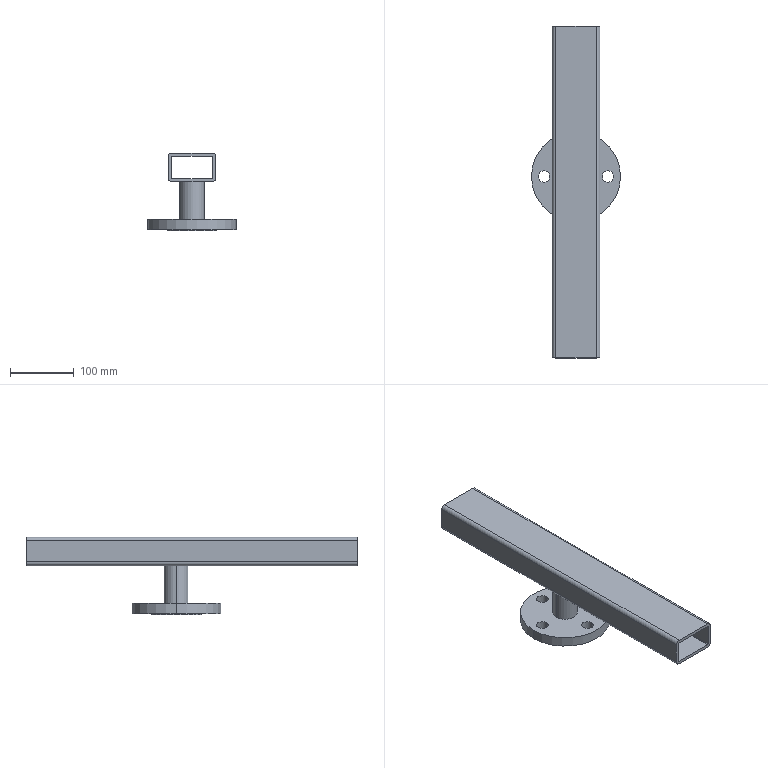Part | SolidWorks | features ICE 4, Extrusion 1 | 2 solids | 38 faces | box 140 x 521 x 122 mm | volume 862843 mm3 | cylinder 24 | plane 14 | commonest cylinder face diameters 18 x8 2 x4 12 x4 38 x2 39 x2 78 x2
STEP:
#1=CARTESIAN_POINT('',(-31.5,285.,-114.722));
#2=VERTEX_POINT('',#1);
#3=CARTESIAN_POINT('',(6.5,285.,-114.722));
#4=VERTEX_POINT('',#3);
#5=CARTESIAN_POINT('',(-12.5,285.,-114.722));
#6=DIRECTION('',(0.,0.,-1.));
#7=DIRECTION('',(-1.,0.,0.));
#8=AXIS2_PLACEMENT_3D('',#5,#6,#7);
#9=CIRCLE('',#8,19.);
#10=EDGE_CURVE('',#2,#4,#9,.T.);
#11=ORIENTED_EDGE('',*,*,#10,.F.);
#12=CARTESIAN_POINT('',(-31.5,285.,-37.722));
#13=VERTEX_POINT('',#12);
#14=CARTESIAN_POINT('',(-31.5,285.,-112.722));
#15=DIRECTION('',(0.,0.,1.));
#16=VECTOR('',#15,1000.);
#17=LINE('',#14,#16);
#18=EDGE_CURVE('',#2,#13,#17,.T.);
#19=ORIENTED_EDGE('',*,*,#18,.T.);
#20=CARTESIAN_POINT('',(6.5,285.,-37.722));
#21=VERTEX_POINT('',#20);
#22=CARTESIAN_POINT('',(-12.5,285.,-37.722));
#23=DIRECTION('',(0.,0.,-1.));
#24=DIRECTION('',(1.,0.,0.));
#25=AXIS2_PLACEMENT_3D('',#22,#23,#24);
#26=CIRCLE('',#25,19.);
#27=EDGE_CURVE('',#13,#21,#26,.T.);
#28=ORIENTED_EDGE('',*,*,#27,.T.);
#29=CARTESIAN_POINT('',(6.5,285.,-112.722));
#30=DIRECTION('',(0.,0.,1.));
#31=VECTOR('',#30,1000.);
#32=LINE('',#29,#31);
#33=EDGE_CURVE('',#4,#21,#32,.T.);
#34=ORIENTED_EDGE('',*,*,#33,.F.);
#35=EDGE_LOOP('',(#11,#19,#28,#34));
#36=FACE_OUTER_BOUND('',#35,.T.);
#37=CARTESIAN_POINT('',(-12.5,285.,-112.722));
#38=DIRECTION('',(0.,0.,1.));
#39=DIRECTION('',(1.,0.,0.));
#40=AXIS2_PLACEMENT_3D('',#37,#38,#39);
#41=CYLINDRICAL_SURFACE('',#40,19.);
#42=ADVANCED_FACE('',(#36),#41,.T.);
#43=CARTESIAN_POINT('',(-12.5,285.,-37.722));
#44=DIRECTION('',(0.,0.,-1.));
#45=DIRECTION('',(1.,0.,0.));
#46=AXIS2_PLACEMENT_3D('',#43,#44,#45);
#47=CIRCLE('',#46,19.);
#48=EDGE_CURVE('',#21,#13,#47,.T.);
#49=ORIENTED_EDGE('',*,*,#48,.F.);
#50=ORIENTED_EDGE('',*,*,#27,.F.);
#51=EDGE_LOOP('',(#49,#50));
#52=FACE_BOUND('',#51,.T.);
#53=CARTESIAN_POINT('',(19.,0.,-37.722));
#54=VERTEX_POINT('',#53);
#55=CARTESIAN_POINT('',(-44.,0.,-37.722));
#56=VERTEX_POINT('',#55);
#57=CARTESIAN_POINT('',(-44.,0.,-37.722));
#58=DIRECTION('',(-1.,0.,0.));
#59=VECTOR('',#58,1000.);
#60=LINE('',#57,#59);
#61=EDGE_CURVE('',#54,#56,#60,.T.);
#62=ORIENTED_EDGE('',*,*,#61,.T.);
#63=CARTESIAN_POINT('',(-44.,521.,-37.722));
#64=VERTEX_POINT('',#63);
#65=CARTESIAN_POINT('',(-44.,521.,-37.722));
#66=DIRECTION('',(0.,-1.,0.));
#67=VECTOR('',#66,1000.);
#68=LINE('',#65,#67);
#69=EDGE_CURVE('',#64,#56,#68,.T.);
#70=ORIENTED_EDGE('',*,*,#69,.F.);
#71=CARTESIAN_POINT('',(19.,521.,-37.722));
#72=VERTEX_POINT('',#71);
#73=CARTESIAN_POINT('',(-44.,521.,-37.722));
#74=DIRECTION('',(-1.,0.,0.));
#75=VECTOR('',#74,1000.);
#76=LINE('',#73,#75);
#77=EDGE_CURVE('',#72,#64,#76,.T.);
#78=ORIENTED_EDGE('',*,*,#77,.F.);
#79=CARTESIAN_POINT('',(19.,521.,-37.722));
#80=DIRECTION('',(0.,-1.,0.));
#81=VECTOR('',#80,1000.);
#82=LINE('',#79,#81);
#83=EDGE_CURVE('',#72,#54,#82,.T.);
#84=ORIENTED_EDGE('',*,*,#83,.T.);
#85=EDGE_LOOP('',(#62,#70,#78,#84));
#86=FACE_OUTER_BOUND('',#85,.T.);
#87=CARTESIAN_POINT('',(-44.,521.,-37.722));
#88=DIRECTION('',(0.,0.,1.));
#89=DIRECTION('',(1.,0.,0.));
#90=AXIS2_PLACEMENT_3D('',#87,#88,#89);
#91=PLANE('',#90);
#92=ADVANCED_FACE('',(#52,#86),#91,.F.);
#93=ORIENTED_EDGE('',*,*,#18,.F.);
#94=CARTESIAN_POINT('',(-12.5,285.,-114.722));
#95=DIRECTION('',(0.,0.,-1.));
#96=DIRECTION('',(-1.,0.,0.));
#97=AXIS2_PLACEMENT_3D('',#94,#95,#96);
#98=CIRCLE('',#97,19.);
#99=EDGE_CURVE('',#4,#2,#98,.T.);
#100=ORIENTED_EDGE('',*,*,#99,.F.);
#101=ORIENTED_EDGE('',*,*,#33,.T.);
#102=ORIENTED_EDGE('',*,*,#48,.T.);
#103=EDGE_LOOP('',(#93,#100,#101,#102));
#104=FACE_OUTER_BOUND('',#103,.T.);
#105=CARTESIAN_POINT('',(-12.5,285.,-112.722));
#106=DIRECTION('',(0.,0.,1.));
#107=DIRECTION('',(1.,0.,0.));
#108=AXIS2_PLACEMENT_3D('',#105,#106,#107);
#109=CYLINDRICAL_SURFACE('',#108,19.);
#110=ADVANCED_FACE('',(#104),#109,.T.);
#111=CARTESIAN_POINT('',(-50.,521.,1.278));
#112=VERTEX_POINT('',#111);
#113=CARTESIAN_POINT('',(-44.,521.,7.278));
#114=VERTEX_POINT('',#113);
#115=CARTESIAN_POINT('',(-44.,521.,1.278));
#116=DIRECTION('',(0.,1.,0.));
#117=DIRECTION('',(0.,0.,-1.));
#118=AXIS2_PLACEMENT_3D('',#115,#116,#117);
#119=CIRCLE('',#118,6.);
#120=EDGE_CURVE('',#112,#114,#119,.T.);
#121=ORIENTED_EDGE('',*,*,#120,.T.);
#122=CARTESIAN_POINT('',(19.,521.,7.278));
#123=VERTEX_POINT('',#122);
#124=CARTESIAN_POINT('',(-44.,521.,7.278));
#125=DIRECTION('',(1.,0.,0.));
#126=VECTOR('',#125,1000.);
#127=LINE('',#124,#126);
#128=EDGE_CURVE('',#114,#123,#127,.T.);
#129=ORIENTED_EDGE('',*,*,#128,.T.);
#130=CARTESIAN_POINT('',(25.,521.,1.278));
#131=VERTEX_POINT('',#130);
#132=CARTESIAN_POINT('',(19.,521.,1.278));
#133=DIRECTION('',(0.,1.,0.));
#134=DIRECTION('',(0.,0.,1.));
#135=AXIS2_PLACEMENT_3D('',#132,#133,#134);
#136=CIRCLE('',#135,6.);
#137=EDGE_CURVE('',#123,#131,#136,.T.);
#138=ORIENTED_EDGE('',*,*,#137,.T.);
#139=CARTESIAN_POINT('',(25.,521.,-31.722));
#140=VERTEX_POINT('',#139);
#141=CARTESIAN_POINT('',(25.,521.,1.278));
#142=DIRECTION('',(0.,0.,-1.));
#143=VECTOR('',#142,1000.);
#144=LINE('',#141,#143);
#145=EDGE_CURVE('',#131,#140,#144,.T.);
#146=ORIENTED_EDGE('',*,*,#145,.T.);
#147=CARTESIAN_POINT('',(19.,521.,-31.722));
#148=DIRECTION('',(0.,1.,0.));
#149=DIRECTION('',(0.,0.,-1.));
#150=AXIS2_PLACEMENT_3D('',#147,#148,#149);
#151=CIRCLE('',#150,6.);
#152=EDGE_CURVE('',#140,#72,#151,.T.);
#153=ORIENTED_EDGE('',*,*,#152,.T.);
#154=ORIENTED_EDGE('',*,*,#77,.T.);
#155=CARTESIAN_POINT('',(-50.,521.,-31.722));
#156=VERTEX_POINT('',#155);
#157=CARTESIAN_POINT('',(-44.,521.,-31.722));
#158=DIRECTION('',(0.,1.,0.));
#159=DIRECTION('',(0.,0.,-1.));
#160=AXIS2_PLACEMENT_3D('',#157,#158,#159);
#161=CIRCLE('',#160,6.);
#162=EDGE_CURVE('',#64,#156,#161,.T.);
#163=ORIENTED_EDGE('',*,*,#162,.T.);
#164=CARTESIAN_POINT('',(-50.,521.,1.278));
#165=DIRECTION('',(0.,0.,1.));
#166=VECTOR('',#165,1000.);
#167=LINE('',#164,#166);
#168=EDGE_CURVE('',#156,#112,#167,.T.);
#169=ORIENTED_EDGE('',*,*,#168,.T.);
#170=EDGE_LOOP('',(#121,#129,#138,#146,#153,#154,#163,#169));
#171=FACE_OUTER_BOUND('',#170,.T.);
#172=CARTESIAN_POINT('',(-45.,521.,1.278));
#173=VERTEX_POINT('',#172);
#174=CARTESIAN_POINT('',(-44.,521.,2.278));
#175=VERTEX_POINT('',#174);
#176=CARTESIAN_POINT('',(-44.,521.,1.278));
#177=DIRECTION('',(0.,1.,0.));
#178=DIRECTION('',(0.,0.,-1.));
#179=AXIS2_PLACEMENT_3D('',#176,#177,#178);
#180=CIRCLE('',#179,1.);
#181=EDGE_CURVE('',#173,#175,#180,.T.);
#182=ORIENTED_EDGE('',*,*,#181,.F.);
#183=CARTESIAN_POINT('',(-45.,521.,-31.722));
#184=VERTEX_POINT('',#183);
#185=CARTESIAN_POINT('',(-45.,521.,1.278));
#186=DIRECTION('',(0.,0.,1.));
#187=VECTOR('',#186,1000.);
#188=LINE('',#185,#187);
#189=EDGE_CURVE('',#184,#173,#188,.T.);
#190=ORIENTED_EDGE('',*,*,#189,.F.);
#191=CARTESIAN_POINT('',(-44.,521.,-32.722));
#192=VERTEX_POINT('',#191);
#193=CARTESIAN_POINT('',(-44.,521.,-31.722));
#194=DIRECTION('',(0.,1.,0.));
#195=DIRECTION('',(0.,0.,-1.));
#196=AXIS2_PLACEMENT_3D('',#193,#194,#195);
#197=CIRCLE('',#196,1.);
#198=EDGE_CURVE('',#192,#184,#197,.T.);
#199=ORIENTED_EDGE('',*,*,#198,.F.);
#200=CARTESIAN_POINT('',(19.,521.,-32.722));
#201=VERTEX_POINT('',#200);
#202=CARTESIAN_POINT('',(-44.,521.,-32.722));
#203=DIRECTION('',(-1.,0.,0.));
#204=VECTOR('',#203,1000.);
#205=LINE('',#202,#204);
#206=EDGE_CURVE('',#201,#192,#205,.T.);
#207=ORIENTED_EDGE('',*,*,#206,.F.);
#208=CARTESIAN_POINT('',(20.,521.,-31.722));
#209=VERTEX_POINT('',#208);
#210=CARTESIAN_POINT('',(19.,521.,-31.722));
#211=DIRECTION('',(0.,1.,0.));
#212=DIRECTION('',(0.,0.,-1.));
#213=AXIS2_PLACEMENT_3D('',#210,#211,#212);
#214=CIRCLE('',#213,1.);
#215=EDGE_CURVE('',#209,#201,#214,.T.);
#216=ORIENTED_EDGE('',*,*,#215,.F.);
#217=CARTESIAN_POINT('',(20.,521.,1.278));
#218=VERTEX_POINT('',#217);
#219=CARTESIAN_POINT('',(20.,521.,1.278));
#220=DIRECTION('',(0.,0.,-1.));
#221=VECTOR('',#220,1000.);
#222=LINE('',#219,#221);
#223=EDGE_CURVE('',#218,#209,#222,.T.);
#224=ORIENTED_EDGE('',*,*,#223,.F.);
#225=CARTESIAN_POINT('',(19.,521.,2.278));
#226=VERTEX_POINT('',#225);
#227=CARTESIAN_POINT('',(19.,521.,1.278));
#228=DIRECTION('',(0.,1.,0.));
#229=DIRECTION('',(0.,0.,1.));
#230=AXIS2_PLACEMENT_3D('',#227,#228,#229);
#231=CIRCLE('',#230,1.);
#232=EDGE_CURVE('',#226,#218,#231,.T.);
#233=ORIENTED_EDGE('',*,*,#232,.F.);
#234=CARTESIAN_POINT('',(-44.,521.,2.278));
#235=DIRECTION('',(1.,0.,0.));
#236=VECTOR('',#235,1000.);
#237=LINE('',#234,#236);
#238=EDGE_CURVE('',#175,#226,#237,.T.);
#239=ORIENTED_EDGE('',*,*,#238,.F.);
#240=EDGE_LOOP('',(#182,#190,#199,#207,#216,#224,#233,#239));
#241=FACE_BOUND('',#240,.T.);
#242=CARTESIAN_POINT('',(-44.,521.,1.278));
#243=DIRECTION('',(0.,-1.,0.));
#244=DIRECTION('',(0.,0.,-1.));
#245=AXIS2_PLACEMENT_3D('',#242,#243,#244);
#246=PLANE('',#245);
#247=ADVANCED_FACE('',(#171,#241),#246,.F.);
#248=CARTESIAN_POINT('',(-50.,0.,1.278));
#249=VERTEX_POINT('',#248);
#250=CARTESIAN_POINT('',(-44.,0.,7.278));
#251=VERTEX_POINT('',#250);
#252=CARTESIAN_POINT('',(-44.,0.,1.278));
#253=DIRECTION('',(0.,1.,0.));
#254=DIRECTION('',(0.,0.,-1.));
#255=AXIS2_PLACEMENT_3D('',#252,#253,#254);
#256=CIRCLE('',#255,6.);
#257=EDGE_CURVE('',#249,#251,#256,.T.);
#258=ORIENTED_EDGE('',*,*,#257,.F.);
#259=CARTESIAN_POINT('',(-50.,0.,-31.722));
#260=VERTEX_POINT('',#259);
#261=CARTESIAN_POINT('',(-50.,0.,1.278));
#262=DIRECTION('',(0.,0.,1.));
#263=VECTOR('',#262,1000.);
#264=LINE('',#261,#263);
#265=EDGE_CURVE('',#260,#249,#264,.T.);
#266=ORIENTED_EDGE('',*,*,#265,.F.);
#267=CARTESIAN_POINT('',(-44.,0.,-31.722));
#268=DIRECTION('',(0.,1.,0.));
#269=DIRECTION('',(0.,0.,-1.));
#270=AXIS2_PLACEMENT_3D('',#267,#268,#269);
#271=CIRCLE('',#270,6.);
#272=EDGE_CURVE('',#56,#260,#271,.T.);
#273=ORIENTED_EDGE('',*,*,#272,.F.);
#274=ORIENTED_EDGE('',*,*,#61,.F.);
#275=CARTESIAN_POINT('',(25.,0.,-31.722));
#276=VERTEX_POINT('',#275);
#277=CARTESIAN_POINT('',(19.,0.,-31.722));
#278=DIRECTION('',(0.,1.,0.));
#279=DIRECTION('',(0.,0.,-1.));
#280=AXIS2_PLACEMENT_3D('',#277,#278,#279);
#281=CIRCLE('',#280,6.);
#282=EDGE_CURVE('',#276,#54,#281,.T.);
#283=ORIENTED_EDGE('',*,*,#282,.F.);
#284=CARTESIAN_POINT('',(25.,0.,1.278));
#285=VERTEX_POINT('',#284);
#286=CARTESIAN_POINT('',(25.,0.,1.278));
#287=DIRECTION('',(0.,0.,-1.));
#288=VECTOR('',#287,1000.);
#289=LINE('',#286,#288);
#290=EDGE_CURVE('',#285,#276,#289,.T.);
#291=ORIENTED_EDGE('',*,*,#290,.F.);
#292=CARTESIAN_POINT('',(19.,0.,7.278));
#293=VERTEX_POINT('',#292);
#294=CARTESIAN_POINT('',(19.,0.,1.278));
#295=DIRECTION('',(0.,1.,0.));
#296=DIRECTION('',(0.,0.,1.));
#297=AXIS2_PLACEMENT_3D('',#294,#295,#296);
#298=CIRCLE('',#297,6.);
#299=EDGE_CURVE('',#293,#285,#298,.T.);
#300=ORIENTED_EDGE('',*,*,#299,.F.);
#301=CARTESIAN_POINT('',(-44.,0.,7.278));
#302=DIRECTION('',(1.,0.,0.));
#303=VECTOR('',#302,1000.);
#304=LINE('',#301,#303);
#305=EDGE_CURVE('',#251,#293,#304,.T.);
#306=ORIENTED_EDGE('',*,*,#305,.F.);
#307=EDGE_LOOP('',(#258,#266,#273,#274,#283,#291,#300,#306));
#308=FACE_OUTER_BOUND('',#307,.T.);
#309=CARTESIAN_POINT('',(-45.,0.,-31.722));
#310=VERTEX_POINT('',#309);
#311=CARTESIAN_POINT('',(-45.,0.,1.278));
#312=VERTEX_POINT('',#311);
#313=CARTESIAN_POINT('',(-45.,0.,1.278));
#314=DIRECTION('',(0.,0.,1.));
#315=VECTOR('',#314,1000.);
#316=LINE('',#313,#315);
#317=EDGE_CURVE('',#310,#312,#316,.T.);
#318=ORIENTED_EDGE('',*,*,#317,.T.);
#319=CARTESIAN_POINT('',(-44.,0.,2.278));
#320=VERTEX_POINT('',#319);
#321=CARTESIAN_POINT('',(-44.,0.,1.278));
#322=DIRECTION('',(0.,1.,0.));
#323=DIRECTION('',(0.,0.,-1.));
#324=AXIS2_PLACEMENT_3D('',#321,#322,#323);
#325=CIRCLE('',#324,1.);
#326=EDGE_CURVE('',#312,#320,#325,.T.);
#327=ORIENTED_EDGE('',*,*,#326,.T.);
#328=CARTESIAN_POINT('',(19.,0.,2.278));
#329=VERTEX_POINT('',#328);
#330=CARTESIAN_POINT('',(-44.,0.,2.278));
#331=DIRECTION('',(1.,0.,0.));
#332=VECTOR('',#331,1000.);
#333=LINE('',#330,#332);
#334=EDGE_CURVE('',#320,#329,#333,.T.);
#335=ORIENTED_EDGE('',*,*,#334,.T.);
#336=CARTESIAN_POINT('',(20.,0.,1.278));
#337=VERTEX_POINT('',#336);
#338=CARTESIAN_POINT('',(19.,0.,1.278));
#339=DIRECTION('',(0.,1.,0.));
#340=DIRECTION('',(0.,0.,1.));
#341=AXIS2_PLACEMENT_3D('',#338,#339,#340);
#342=CIRCLE('',#341,1.);
#343=EDGE_CURVE('',#329,#337,#342,.T.);
#344=ORIENTED_EDGE('',*,*,#343,.T.);
#345=CARTESIAN_POINT('',(20.,0.,-31.722));
#346=VERTEX_POINT('',#345);
#347=CARTESIAN_POINT('',(20.,0.,1.278));
#348=DIRECTION('',(0.,0.,-1.));
#349=VECTOR('',#348,1000.);
#350=LINE('',#347,#349);
#351=EDGE_CURVE('',#337,#346,#350,.T.);
#352=ORIENTED_EDGE('',*,*,#351,.T.);
#353=CARTESIAN_POINT('',(19.,0.,-32.722));
#354=VERTEX_POINT('',#353);
#355=CARTESIAN_POINT('',(19.,0.,-31.722));
#356=DIRECTION('',(0.,1.,0.));
#357=DIRECTION('',(0.,0.,-1.));
#358=AXIS2_PLACEMENT_3D('',#355,#356,#357);
#359=CIRCLE('',#358,1.);
#360=EDGE_CURVE('',#346,#354,#359,.T.);
#361=ORIENTED_EDGE('',*,*,#360,.T.);
#362=CARTESIAN_POINT('',(-44.,0.,-32.722));
#363=VERTEX_POINT('',#362);
#364=CARTESIAN_POINT('',(-44.,0.,-32.722));
#365=DIRECTION('',(-1.,0.,0.));
#366=VECTOR('',#365,1000.);
#367=LINE('',#364,#366);
#368=EDGE_CURVE('',#354,#363,#367,.T.);
#369=ORIENTED_EDGE('',*,*,#368,.T.);
#370=CARTESIAN_POINT('',(-44.,0.,-31.722));
#371=DIRECTION('',(0.,1.,0.));
#372=DIRECTION('',(0.,0.,-1.));
#373=AXIS2_PLACEMENT_3D('',#370,#371,#372);
#374=CIRCLE('',#373,1.);
#375=EDGE_CURVE('',#363,#310,#374,.T.);
#376=ORIENTED_EDGE('',*,*,#375,.T.);
#377=EDGE_LOOP('',(#318,#327,#335,#344,#352,#361,#369,#376));
#378=FACE_BOUND('',#377,.T.);
#379=CARTESIAN_POINT('',(-44.,0.,1.278));
#380=DIRECTION('',(0.,-1.,0.));
#381=DIRECTION('',(0.,0.,-1.));
#382=AXIS2_PLACEMENT_3D('',#379,#380,#381);
#383=PLANE('',#382);
#384=ADVANCED_FACE('',(#308,#378),#383,.T.);
#385=ORIENTED_EDGE('',*,*,#257,.T.);
#386=CARTESIAN_POINT('',(-44.,521.,7.278));
#387=DIRECTION('',(0.,-1.,0.));
#388=VECTOR('',#387,1000.);
#389=LINE('',#386,#388);
#390=EDGE_CURVE('',#114,#251,#389,.T.);
#391=ORIENTED_EDGE('',*,*,#390,.F.);
#392=ORIENTED_EDGE('',*,*,#120,.F.);
#393=CARTESIAN_POINT('',(-50.,521.,1.278));
#394=DIRECTION('',(0.,-1.,0.));
#395=VECTOR('',#394,1000.);
#396=LINE('',#393,#395);
#397=EDGE_CURVE('',#112,#249,#396,.T.);
#398=ORIENTED_EDGE('',*,*,#397,.T.);
#399=EDGE_LOOP('',(#385,#391,#392,#398));
#400=FACE_OUTER_BOUND('',#399,.T.);
#401=CARTESIAN_POINT('',(-44.,521.,1.278));
#402=DIRECTION('',(0.,-1.,0.));
#403=DIRECTION('',(0.,0.,-1.));
#404=AXIS2_PLACEMENT_3D('',#401,#402,#403);
#405=CYLINDRICAL_SURFACE('',#404,6.);
#406=ADVANCED_FACE('',(#400),#405,.T.);
#407=ORIENTED_EDGE('',*,*,#305,.T.);
#408=CARTESIAN_POINT('',(19.,521.,7.278));
#409=DIRECTION('',(0.,-1.,0.));
#410=VECTOR('',#409,1000.);
#411=LINE('',#408,#410);
#412=EDGE_CURVE('',#123,#293,#411,.T.);
#413=ORIENTED_EDGE('',*,*,#412,.F.);
#414=ORIENTED_EDGE('',*,*,#128,.F.);
#415=ORIENTED_EDGE('',*,*,#390,.T.);
#416=EDGE_LOOP('',(#407,#413,#414,#415));
#417=FACE_OUTER_BOUND('',#416,.T.);
#418=CARTESIAN_POINT('',(-44.,521.,7.278));
#419=DIRECTION('',(0.,0.,-1.));
#420=DIRECTION('',(-1.,0.,0.));
#421=AXIS2_PLACEMENT_3D('',#418,#419,#420);
#422=PLANE('',#421);
#423=ADVANCED_FACE('',(#417),#422,.F.);
#424=ORIENTED_EDGE('',*,*,#299,.T.);
#425=CARTESIAN_POINT('',(25.,521.,1.278));
#426=DIRECTION('',(0.,-1.,0.));
#427=VECTOR('',#426,1000.);
#428=LINE('',#425,#427);
#429=EDGE_CURVE('',#131,#285,#428,.T.);
#430=ORIENTED_EDGE('',*,*,#429,.F.);
#431=ORIENTED_EDGE('',*,*,#137,.F.);
#432=ORIENTED_EDGE('',*,*,#412,.T.);
#433=EDGE_LOOP('',(#424,#430,#431,#432));
#434=FACE_OUTER_BOUND('',#433,.T.);
#435=CARTESIAN_POINT('',(19.,521.,1.278));
#436=DIRECTION('',(0.,-1.,0.));
#437=DIRECTION('',(0.,0.,-1.));
#438=AXIS2_PLACEMENT_3D('',#435,#436,#437);
#439=CYLINDRICAL_SURFACE('',#438,6.);
#440=ADVANCED_FACE('',(#434),#439,.T.);
#441=ORIENTED_EDGE('',*,*,#290,.T.);
#442=CARTESIAN_POINT('',(25.,521.,-31.722));
#443=DIRECTION('',(0.,-1.,0.));
#444=VECTOR('',#443,1000.);
#445=LINE('',#442,#444);
#446=EDGE_CURVE('',#140,#276,#445,.T.);
#447=ORIENTED_EDGE('',*,*,#446,.F.);
#448=ORIENTED_EDGE('',*,*,#145,.F.);
#449=ORIENTED_EDGE('',*,*,#429,.T.);
#450=EDGE_LOOP('',(#441,#447,#448,#449));
#451=FACE_OUTER_BOUND('',#450,.T.);
#452=CARTESIAN_POINT('',(25.,521.,1.278));
#453=DIRECTION('',(-1.,0.,0.));
#454=DIRECTION('',(0.,0.,1.));
#455=AXIS2_PLACEMENT_3D('',#452,#453,#454);
#456=PLANE('',#455);
#457=ADVANCED_FACE('',(#451),#456,.F.);
#458=ORIENTED_EDGE('',*,*,#282,.T.);
#459=ORIENTED_EDGE('',*,*,#83,.F.);
#460=ORIENTED_EDGE('',*,*,#152,.F.);
#461=ORIENTED_EDGE('',*,*,#446,.T.);
#462=EDGE_LOOP('',(#458,#459,#460,#461));
#463=FACE_OUTER_BOUND('',#462,.T.);
#464=CARTESIAN_POINT('',(19.,521.,-31.722));
#465=DIRECTION('',(0.,-1.,0.));
#466=DIRECTION('',(0.,0.,-1.));
#467=AXIS2_PLACEMENT_3D('',#464,#465,#466);
#468=CYLINDRICAL_SURFACE('',#467,6.);
#469=ADVANCED_FACE('',(#463),#468,.T.);
#470=ORIENTED_EDGE('',*,*,#272,.T.);
#471=CARTESIAN_POINT('',(-50.,521.,-31.722));
#472=DIRECTION('',(0.,-1.,0.));
#473=VECTOR('',#472,1000.);
#474=LINE('',#471,#473);
#475=EDGE_CURVE('',#156,#260,#474,.T.);
#476=ORIENTED_EDGE('',*,*,#475,.F.);
#477=ORIENTED_EDGE('',*,*,#162,.F.);
#478=ORIENTED_EDGE('',*,*,#69,.T.);
#479=EDGE_LOOP('',(#470,#476,#477,#478));
#480=FACE_OUTER_BOUND('',#479,.T.);
#481=CARTESIAN_POINT('',(-44.,521.,-31.722));
#482=DIRECTION('',(0.,-1.,0.));
#483=DIRECTION('',(0.,0.,-1.));
#484=AXIS2_PLACEMENT_3D('',#481,#482,#483);
#485=CYLINDRICAL_SURFACE('',#484,6.);
#486=ADVANCED_FACE('',(#480),#485,.T.);
#487=ORIENTED_EDGE('',*,*,#265,.T.);
#488=ORIENTED_EDGE('',*,*,#397,.F.);
#489=ORIENTED_EDGE('',*,*,#168,.F.);
#490=ORIENTED_EDGE('',*,*,#475,.T.);
#491=EDGE_LOOP('',(#487,#488,#489,#490));
#492=FACE_OUTER_BOUND('',#491,.T.);
#493=CARTESIAN_POINT('',(-50.,521.,1.278));
#494=DIRECTION('',(1.,0.,0.));
#495=DIRECTION('',(0.,0.,-1.));
#496=AXIS2_PLACEMENT_3D('',#493,#494,#495);
#497=PLANE('',#496);
#498=ADVANCED_FACE('',(#492),#497,.F.);
#499=ORIENTED_EDGE('',*,*,#326,.F.);
#500=CARTESIAN_POINT('',(-45.,521.,1.278));
#501=DIRECTION('',(0.,-1.,0.));
#502=VECTOR('',#501,1000.);
#503=LINE('',#500,#502);
#504=EDGE_CURVE('',#173,#312,#503,.T.);
#505=ORIENTED_EDGE('',*,*,#504,.F.);
#506=ORIENTED_EDGE('',*,*,#181,.T.);
#507=CARTESIAN_POINT('',(-44.,521.,2.278));
#508=DIRECTION('',(0.,-1.,0.));
#509=VECTOR('',#508,1000.);
#510=LINE('',#507,#509);
#511=EDGE_CURVE('',#175,#320,#510,.T.);
#512=ORIENTED_EDGE('',*,*,#511,.T.);
#513=EDGE_LOOP('',(#499,#505,#506,#512));
#514=FACE_OUTER_BOUND('',#513,.T.);
#515=CARTESIAN_POINT('',(-44.,521.,1.278));
#516=DIRECTION('',(0.,-1.,0.));
#517=DIRECTION('',(0.,0.,-1.));
#518=AXIS2_PLACEMENT_3D('',#515,#516,#517);
#519=CYLINDRICAL_SURFACE('',#518,1.);
#520=ADVANCED_FACE('',(#514),#519,.F.);
#521=ORIENTED_EDGE('',*,*,#334,.F.);
#522=ORIENTED_EDGE('',*,*,#511,.F.);
#523=ORIENTED_EDGE('',*,*,#238,.T.);
#524=CARTESIAN_POINT('',(19.,521.,2.278));
#525=DIRECTION('',(0.,-1.,0.));
#526=VECTOR('',#525,1000.);
#527=LINE('',#524,#526);
#528=EDGE_CURVE('',#226,#329,#527,.T.);
#529=ORIENTED_EDGE('',*,*,#528,.T.);
#530=EDGE_LOOP('',(#521,#522,#523,#529));
#531=FACE_OUTER_BOUND('',#530,.T.);
#532=CARTESIAN_POINT('',(-44.,521.,2.278));
#533=DIRECTION('',(0.,0.,-1.));
#534=DIRECTION('',(-1.,0.,0.));
#535=AXIS2_PLACEMENT_3D('',#532,#533,#534);
#536=PLANE('',#535);
#537=ADVANCED_FACE('',(#531),#536,.T.);
#538=ORIENTED_EDGE('',*,*,#343,.F.);
#539=ORIENTED_EDGE('',*,*,#528,.F.);
#540=ORIENTED_EDGE('',*,*,#232,.T.);
#541=CARTESIAN_POINT('',(20.,521.,1.278));
#542=DIRECTION('',(0.,-1.,0.));
#543=VECTOR('',#542,1000.);
#544=LINE('',#541,#543);
#545=EDGE_CURVE('',#218,#337,#544,.T.);
#546=ORIENTED_EDGE('',*,*,#545,.T.);
#547=EDGE_LOOP('',(#538,#539,#540,#546));
#548=FACE_OUTER_BOUND('',#547,.T.);
#549=CARTESIAN_POINT('',(19.,521.,1.278));
#550=DIRECTION('',(0.,-1.,0.));
#551=DIRECTION('',(0.,0.,-1.));
#552=AXIS2_PLACEMENT_3D('',#549,#550,#551);
#553=CYLINDRICAL_SURFACE('',#552,1.);
#554=ADVANCED_FACE('',(#548),#553,.F.);
#555=ORIENTED_EDGE('',*,*,#351,.F.);
#556=ORIENTED_EDGE('',*,*,#545,.F.);
#557=ORIENTED_EDGE('',*,*,#223,.T.);
#558=CARTESIAN_POINT('',(20.,521.,-31.722));
#559=DIRECTION('',(0.,-1.,0.));
#560=VECTOR('',#559,1000.);
#561=LINE('',#558,#560);
#562=EDGE_CURVE('',#209,#346,#561,.T.);
#563=ORIENTED_EDGE('',*,*,#562,.T.);
#564=EDGE_LOOP('',(#555,#556,#557,#563));
#565=FACE_OUTER_BOUND('',#564,.T.);
#566=CARTESIAN_POINT('',(20.,521.,1.278));
#567=DIRECTION('',(-1.,0.,0.));
#568=DIRECTION('',(0.,0.,1.));
#569=AXIS2_PLACEMENT_3D('',#566,#567,#568);
#570=PLANE('',#569);
#571=ADVANCED_FACE('',(#565),#570,.T.);
#572=ORIENTED_EDGE('',*,*,#360,.F.);
#573=ORIENTED_EDGE('',*,*,#562,.F.);
#574=ORIENTED_EDGE('',*,*,#215,.T.);
#575=CARTESIAN_POINT('',(19.,521.,-32.722));
#576=DIRECTION('',(0.,-1.,0.));
#577=VECTOR('',#576,1000.);
#578=LINE('',#575,#577);
#579=EDGE_CURVE('',#201,#354,#578,.T.);
#580=ORIENTED_EDGE('',*,*,#579,.T.);
#581=EDGE_LOOP('',(#572,#573,#574,#580));
#582=FACE_OUTER_BOUND('',#581,.T.);
#583=CARTESIAN_POINT('',(19.,521.,-31.722));
#584=DIRECTION('',(0.,-1.,0.));
#585=DIRECTION('',(0.,0.,-1.));
#586=AXIS2_PLACEMENT_3D('',#583,#584,#585);
#587=CYLINDRICAL_SURFACE('',#586,1.);
#588=ADVANCED_FACE('',(#582),#587,.F.);
#589=ORIENTED_EDGE('',*,*,#368,.F.);
#590=ORIENTED_EDGE('',*,*,#579,.F.);
#591=ORIENTED_EDGE('',*,*,#206,.T.);
#592=CARTESIAN_POINT('',(-44.,521.,-32.722));
#593=DIRECTION('',(0.,-1.,0.));
#594=VECTOR('',#593,1000.);
#595=LINE('',#592,#594);
#596=EDGE_CURVE('',#192,#363,#595,.T.);
#597=ORIENTED_EDGE('',*,*,#596,.T.);
#598=EDGE_LOOP('',(#589,#590,#591,#597));
#599=FACE_OUTER_BOUND('',#598,.T.);
#600=CARTESIAN_POINT('',(-44.,521.,-32.722));
#601=DIRECTION('',(0.,0.,1.));
#602=DIRECTION('',(1.,0.,0.));
#603=AXIS2_PLACEMENT_3D('',#600,#601,#602);
#604=PLANE('',#603);
#605=ADVANCED_FACE('',(#599),#604,.T.);
#606=ORIENTED_EDGE('',*,*,#375,.F.);
#607=ORIENTED_EDGE('',*,*,#596,.F.);
#608=ORIENTED_EDGE('',*,*,#198,.T.);
#609=CARTESIAN_POINT('',(-45.,521.,-31.722));
#610=DIRECTION('',(0.,-1.,0.));
#611=VECTOR('',#610,1000.);
#612=LINE('',#609,#611);
#613=EDGE_CURVE('',#184,#310,#612,.T.);
#614=ORIENTED_EDGE('',*,*,#613,.T.);
#615=EDGE_LOOP('',(#606,#607,#608,#614));
#616=FACE_OUTER_BOUND('',#615,.T.);
#617=CARTESIAN_POINT('',(-44.,521.,-31.722));
#618=DIRECTION('',(0.,-1.,0.));
#619=DIRECTION('',(0.,0.,-1.));
#620=AXIS2_PLACEMENT_3D('',#617,#618,#619);
#621=CYLINDRICAL_SURFACE('',#620,1.);
#622=ADVANCED_FACE('',(#616),#621,.F.);
#623=ORIENTED_EDGE('',*,*,#317,.F.);
#624=ORIENTED_EDGE('',*,*,#613,.F.);
#625=ORIENTED_EDGE('',*,*,#189,.T.);
#626=ORIENTED_EDGE('',*,*,#504,.T.);
#627=EDGE_LOOP('',(#623,#624,#625,#626));
#628=FACE_OUTER_BOUND('',#627,.T.);
#629=CARTESIAN_POINT('',(-45.,521.,1.278));
#630=DIRECTION('',(1.,0.,0.));
#631=DIRECTION('',(0.,0.,-1.));
#632=AXIS2_PLACEMENT_3D('',#629,#630,#631);
#633=PLANE('',#632);
#634=ADVANCED_FACE('',(#628),#633,.T.);
#635=ORIENTED_EDGE('',*,*,#99,.T.);
#636=ORIENTED_EDGE('',*,*,#10,.T.);
#637=EDGE_LOOP('',(#635,#636));
#638=FACE_OUTER_BOUND('',#637,.T.);
#639=CARTESIAN_POINT('',(-12.5,285.,-114.722));
#640=DIRECTION('',(0.,0.,-1.));
#641=DIRECTION('',(-1.,0.,0.));
#642=AXIS2_PLACEMENT_3D('',#639,#640,#641);
#643=PLANE('',#642);
#644=ADVANCED_FACE('',(#638),#643,.T.);
#645=CLOSED_SHELL('',(#42,#92,#110,#247,#384,#406,#423,#440,#457,#469,#486,#498,#520,#537,#554,#571,#588,#605,#622,#634,#644));
#646=MANIFOLD_SOLID_BREP('',#645);
#647=CARTESIAN_POINT('',(7.,285.,-96.722));
#648=VERTEX_POINT('',#647);
#649=CARTESIAN_POINT('',(-32.,285.,-96.722));
#650=VERTEX_POINT('',#649);
#651=CARTESIAN_POINT('',(-12.5,285.,-96.722));
#652=DIRECTION('',(0.,0.,-1.));
#653=DIRECTION('',(-1.,0.,0.));
#654=AXIS2_PLACEMENT_3D('',#651,#652,#653);
#655=CIRCLE('',#654,19.5);
#656=EDGE_CURVE('',#648,#650,#655,.T.);
#657=ORIENTED_EDGE('',*,*,#656,.F.);
#658=CARTESIAN_POINT('',(7.,285.,-114.722));
#659=VERTEX_POINT('',#658);
#660=CARTESIAN_POINT('',(7.,285.,17.432));
#661=DIRECTION('',(0.,0.,-1.));
#662=VECTOR('',#661,1000.);
#663=LINE('',#660,#662);
#664=EDGE_CURVE('',#648,#659,#663,.T.);
#665=ORIENTED_EDGE('',*,*,#664,.T.);
#666=CARTESIAN_POINT('',(-32.,285.,-114.722));
#667=VERTEX_POINT('',#666);
#668=CARTESIAN_POINT('',(-12.5,285.,-114.722));
#669=DIRECTION('',(0.,0.,-1.));
#670=DIRECTION('',(-1.,0.,0.));
#671=AXIS2_PLACEMENT_3D('',#668,#669,#670);
#672=CIRCLE('',#671,19.5);
#673=EDGE_CURVE('',#659,#667,#672,.T.);
#674=ORIENTED_EDGE('',*,*,#673,.T.);
#675=CARTESIAN_POINT('',(-32.,285.,17.432));
#676=DIRECTION('',(0.,0.,-1.));
#677=VECTOR('',#676,1000.);
#678=LINE('',#675,#677);
#679=EDGE_CURVE('',#650,#667,#678,.T.);
#680=ORIENTED_EDGE('',*,*,#679,.F.);
#681=EDGE_LOOP('',(#657,#665,#674,#680));
#682=FACE_OUTER_BOUND('',#681,.T.);
#683=CARTESIAN_POINT('',(-12.5,285.,17.432));
#684=DIRECTION('',(0.,0.,-1.));
#685=DIRECTION('',(-1.,0.,0.));
#686=AXIS2_PLACEMENT_3D('',#683,#684,#685);
#687=CYLINDRICAL_SURFACE('',#686,19.5);
#688=ADVANCED_FACE('',(#682),#687,.F.);
#689=CARTESIAN_POINT('',(-51.5,285.,-114.722));
#690=VERTEX_POINT('',#689);
#691=CARTESIAN_POINT('',(26.5,285.,-114.722));
#692=VERTEX_POINT('',#691);
#693=CARTESIAN_POINT('',(-12.5,285.,-114.722));
#694=DIRECTION('',(0.,0.,-1.));
#695=DIRECTION('',(-1.,0.,0.));
#696=AXIS2_PLACEMENT_3D('',#693,#694,#695);
#697=CIRCLE('',#696,39.);
#698=EDGE_CURVE('',#690,#692,#697,.T.);
#699=ORIENTED_EDGE('',*,*,#698,.F.);
#700=CARTESIAN_POINT('',(-51.5,285.,-112.722));
#701=VERTEX_POINT('',#700);
#702=CARTESIAN_POINT('',(-51.5,285.,-114.722));
#703=DIRECTION('',(0.,0.,1.));
#704=VECTOR('',#703,1000.);
#705=LINE('',#702,#704);
#706=EDGE_CURVE('',#690,#701,#705,.T.);
#707=ORIENTED_EDGE('',*,*,#706,.T.);
#708=CARTESIAN_POINT('',(26.5,285.,-112.722));
#709=VERTEX_POINT('',#708);
#710=CARTESIAN_POINT('',(-12.5,285.,-112.722));
#711=DIRECTION('',(0.,0.,-1.));
#712=DIRECTION('',(-1.,0.,0.));
#713=AXIS2_PLACEMENT_3D('',#710,#711,#712);
#714=CIRCLE('',#713,39.);
#715=EDGE_CURVE('',#701,#709,#714,.T.);
#716=ORIENTED_EDGE('',*,*,#715,.T.);
#717=CARTESIAN_POINT('',(26.5,285.,-114.722));
#718=DIRECTION('',(0.,0.,1.));
#719=VECTOR('',#718,1000.);
#720=LINE('',#717,#719);
#721=EDGE_CURVE('',#692,#709,#720,.T.);
#722=ORIENTED_EDGE('',*,*,#721,.F.);
#723=EDGE_LOOP('',(#699,#707,#716,#722));
#724=FACE_OUTER_BOUND('',#723,.T.);
#725=CARTESIAN_POINT('',(-12.5,285.,-114.722));
#726=DIRECTION('',(0.,0.,1.));
#727=DIRECTION('',(1.,0.,0.));
#728=AXIS2_PLACEMENT_3D('',#725,#726,#727);
#729=CYLINDRICAL_SURFACE('',#728,39.);
#730=ADVANCED_FACE('',(#724),#729,.T.);
#731=CARTESIAN_POINT('',(46.5,285.,-96.722));
#732=VERTEX_POINT('',#731);
#733=CARTESIAN_POINT('',(28.5,285.,-96.722));
#734=VERTEX_POINT('',#733);
#735=CARTESIAN_POINT('',(37.5,285.,-96.722));
#736=DIRECTION('',(0.,0.,-1.));
#737=DIRECTION('',(-1.,0.,0.));
#738=AXIS2_PLACEMENT_3D('',#735,#736,#737);
#739=CIRCLE('',#738,9.);
#740=EDGE_CURVE('',#732,#734,#739,.T.);
#741=ORIENTED_EDGE('',*,*,#740,.F.);
#742=CARTESIAN_POINT('',(46.5,285.,-112.722));
#743=VERTEX_POINT('',#742);
#744=CARTESIAN_POINT('',(46.5,285.,-96.722));
#745=DIRECTION('',(0.,0.,-1.));
#746=VECTOR('',#745,1000.);
#747=LINE('',#744,#746);
#748=EDGE_CURVE('',#732,#743,#747,.T.);
#749=ORIENTED_EDGE('',*,*,#748,.T.);
#750=CARTESIAN_POINT('',(28.5,285.,-112.722));
#751=VERTEX_POINT('',#750);
#752=CARTESIAN_POINT('',(37.5,285.,-112.722));
#753=DIRECTION('',(0.,0.,-1.));
#754=DIRECTION('',(-1.,0.,0.));
#755=AXIS2_PLACEMENT_3D('',#752,#753,#754);
#756=CIRCLE('',#755,9.);
#757=EDGE_CURVE('',#743,#751,#756,.T.);
#758=ORIENTED_EDGE('',*,*,#757,.T.);
#759=CARTESIAN_POINT('',(28.5,285.,-96.722));
#760=DIRECTION('',(0.,0.,-1.));
#761=VECTOR('',#760,1000.);
#762=LINE('',#759,#761);
#763=EDGE_CURVE('',#734,#751,#762,.T.);
#764=ORIENTED_EDGE('',*,*,#763,.F.);
#765=EDGE_LOOP('',(#741,#749,#758,#764));
#766=FACE_OUTER_BOUND('',#765,.T.);
#767=CARTESIAN_POINT('',(37.5,285.,-96.722));
#768=DIRECTION('',(0.,0.,-1.));
#769=DIRECTION('',(-1.,0.,0.));
#770=AXIS2_PLACEMENT_3D('',#767,#768,#769);
#771=CYLINDRICAL_SURFACE('',#770,9.);
#772=ADVANCED_FACE('',(#766),#771,.F.);
#773=CARTESIAN_POINT('',(-3.5,235.,-96.722));
#774=VERTEX_POINT('',#773);
#775=CARTESIAN_POINT('',(-21.5,235.,-96.722));
#776=VERTEX_POINT('',#775);
#777=CARTESIAN_POINT('',(-12.5,235.,-96.722));
#778=DIRECTION('',(0.,0.,-1.));
#779=DIRECTION('',(-1.,0.,0.));
#780=AXIS2_PLACEMENT_3D('',#777,#778,#779);
#781=CIRCLE('',#780,9.);
#782=EDGE_CURVE('',#774,#776,#781,.T.);
#783=ORIENTED_EDGE('',*,*,#782,.F.);
#784=CARTESIAN_POINT('',(-3.5,235.,-112.722));
#785=VERTEX_POINT('',#784);
#786=CARTESIAN_POINT('',(-3.5,235.,-96.722));
#787=DIRECTION('',(0.,0.,-1.));
#788=VECTOR('',#787,1000.);
#789=LINE('',#786,#788);
#790=EDGE_CURVE('',#774,#785,#789,.T.);
#791=ORIENTED_EDGE('',*,*,#790,.T.);
#792=CARTESIAN_POINT('',(-21.5,235.,-112.722));
#793=VERTEX_POINT('',#792);
#794=CARTESIAN_POINT('',(-12.5,235.,-112.722));
#795=DIRECTION('',(0.,0.,-1.));
#796=DIRECTION('',(-1.,0.,0.));
#797=AXIS2_PLACEMENT_3D('',#794,#795,#796);
#798=CIRCLE('',#797,9.);
#799=EDGE_CURVE('',#785,#793,#798,.T.);
#800=ORIENTED_EDGE('',*,*,#799,.T.);
#801=CARTESIAN_POINT('',(-21.5,235.,-96.722));
#802=DIRECTION('',(0.,0.,-1.));
#803=VECTOR('',#802,1000.);
#804=LINE('',#801,#803);
#805=EDGE_CURVE('',#776,#793,#804,.T.);
#806=ORIENTED_EDGE('',*,*,#805,.F.);
#807=EDGE_LOOP('',(#783,#791,#800,#806));
#808=FACE_OUTER_BOUND('',#807,.T.);
#809=CARTESIAN_POINT('',(-12.5,235.,-96.722));
#810=DIRECTION('',(0.,0.,-1.));
#811=DIRECTION('',(-1.,0.,0.));
#812=AXIS2_PLACEMENT_3D('',#809,#810,#811);
#813=CYLINDRICAL_SURFACE('',#812,9.);
#814=ADVANCED_FACE('',(#808),#813,.F.);
#815=CARTESIAN_POINT('',(-53.5,285.,-96.722));
#816=VERTEX_POINT('',#815);
#817=CARTESIAN_POINT('',(-71.5,285.,-96.722));
#818=VERTEX_POINT('',#817);
#819=CARTESIAN_POINT('',(-62.5,285.,-96.722));
#820=DIRECTION('',(0.,0.,-1.));
#821=DIRECTION('',(-1.,0.,0.));
#822=AXIS2_PLACEMENT_3D('',#819,#820,#821);
#823=CIRCLE('',#822,9.);
#824=EDGE_CURVE('',#816,#818,#823,.T.);
#825=ORIENTED_EDGE('',*,*,#824,.F.);
#826=CARTESIAN_POINT('',(-53.5,285.,-112.722));
#827=VERTEX_POINT('',#826);
#828=CARTESIAN_POINT('',(-53.5,285.,-96.722));
#829=DIRECTION('',(0.,0.,-1.));
#830=VECTOR('',#829,1000.);
#831=LINE('',#828,#830);
#832=EDGE_CURVE('',#816,#827,#831,.T.);
#833=ORIENTED_EDGE('',*,*,#832,.T.);
#834=CARTESIAN_POINT('',(-71.5,285.,-112.722));
#835=VERTEX_POINT('',#834);
#836=CARTESIAN_POINT('',(-62.5,285.,-112.722));
#837=DIRECTION('',(0.,0.,-1.));
#838=DIRECTION('',(-1.,0.,0.));
#839=AXIS2_PLACEMENT_3D('',#836,#837,#838);
#840=CIRCLE('',#839,9.);
#841=EDGE_CURVE('',#827,#835,#840,.T.);
#842=ORIENTED_EDGE('',*,*,#841,.T.);
#843=CARTESIAN_POINT('',(-71.5,285.,-96.722));
#844=DIRECTION('',(0.,0.,-1.));
#845=VECTOR('',#844,1000.);
#846=LINE('',#843,#845);
#847=EDGE_CURVE('',#818,#835,#846,.T.);
#848=ORIENTED_EDGE('',*,*,#847,.F.);
#849=EDGE_LOOP('',(#825,#833,#842,#848));
#850=FACE_OUTER_BOUND('',#849,.T.);
#851=CARTESIAN_POINT('',(-62.5,285.,-96.722));
#852=DIRECTION('',(0.,0.,-1.));
#853=DIRECTION('',(-1.,0.,0.));
#854=AXIS2_PLACEMENT_3D('',#851,#852,#853);
#855=CYLINDRICAL_SURFACE('',#854,9.);
#856=ADVANCED_FACE('',(#850),#855,.F.);
#857=CARTESIAN_POINT('',(-3.5,335.,-96.722));
#858=VERTEX_POINT('',#857);
#859=CARTESIAN_POINT('',(-21.5,335.,-96.722));
#860=VERTEX_POINT('',#859);
#861=CARTESIAN_POINT('',(-12.5,335.,-96.722));
#862=DIRECTION('',(0.,0.,-1.));
#863=DIRECTION('',(-1.,0.,0.));
#864=AXIS2_PLACEMENT_3D('',#861,#862,#863);
#865=CIRCLE('',#864,9.);
#866=EDGE_CURVE('',#858,#860,#865,.T.);
#867=ORIENTED_EDGE('',*,*,#866,.F.);
#868=CARTESIAN_POINT('',(-3.5,335.,-112.722));
#869=VERTEX_POINT('',#868);
#870=CARTESIAN_POINT('',(-3.5,335.,-96.722));
#871=DIRECTION('',(0.,0.,-1.));
#872=VECTOR('',#871,1000.);
#873=LINE('',#870,#872);
#874=EDGE_CURVE('',#858,#869,#873,.T.);
#875=ORIENTED_EDGE('',*,*,#874,.T.);
#876=CARTESIAN_POINT('',(-21.5,335.,-112.722));
#877=VERTEX_POINT('',#876);
#878=CARTESIAN_POINT('',(-12.5,335.,-112.722));
#879=DIRECTION('',(0.,0.,-1.));
#880=DIRECTION('',(-1.,0.,0.));
#881=AXIS2_PLACEMENT_3D('',#878,#879,#880);
#882=CIRCLE('',#881,9.);
#883=EDGE_CURVE('',#869,#877,#882,.T.);
#884=ORIENTED_EDGE('',*,*,#883,.T.);
#885=CARTESIAN_POINT('',(-21.5,335.,-96.722));
#886=DIRECTION('',(0.,0.,-1.));
#887=VECTOR('',#886,1000.);
#888=LINE('',#885,#887);
#889=EDGE_CURVE('',#860,#877,#888,.T.);
#890=ORIENTED_EDGE('',*,*,#889,.F.);
#891=EDGE_LOOP('',(#867,#875,#884,#890));
#892=FACE_OUTER_BOUND('',#891,.T.);
#893=CARTESIAN_POINT('',(-12.5,335.,-96.722));
#894=DIRECTION('',(0.,0.,-1.));
#895=DIRECTION('',(-1.,0.,0.));
#896=AXIS2_PLACEMENT_3D('',#893,#894,#895);
#897=CYLINDRICAL_SURFACE('',#896,9.);
#898=ADVANCED_FACE('',(#892),#897,.F.);
#899=CARTESIAN_POINT('',(-82.5,285.,-96.722));
#900=VERTEX_POINT('',#899);
#901=CARTESIAN_POINT('',(57.5,285.,-96.722));
#902=VERTEX_POINT('',#901);
#903=CARTESIAN_POINT('',(-12.5,285.,-96.722));
#904=DIRECTION('',(0.,0.,-1.));
#905=DIRECTION('',(-1.,0.,0.));
#906=AXIS2_PLACEMENT_3D('',#903,#904,#905);
#907=CIRCLE('',#906,70.);
#908=EDGE_CURVE('',#900,#902,#907,.T.);
#909=ORIENTED_EDGE('',*,*,#908,.T.);
#910=CARTESIAN_POINT('',(57.5,285.,-112.722));
#911=VERTEX_POINT('',#910);
#912=CARTESIAN_POINT('',(57.5,285.,-96.722));
#913=DIRECTION('',(0.,0.,-1.));
#914=VECTOR('',#913,1000.);
#915=LINE('',#912,#914);
#916=EDGE_CURVE('',#902,#911,#915,.T.);
#917=ORIENTED_EDGE('',*,*,#916,.T.);
#918=CARTESIAN_POINT('',(-82.5,285.,-112.722));
#919=VERTEX_POINT('',#918);
#920=CARTESIAN_POINT('',(-12.5,285.,-112.722));
#921=DIRECTION('',(0.,0.,-1.));
#922=DIRECTION('',(-1.,0.,0.));
#923=AXIS2_PLACEMENT_3D('',#920,#921,#922);
#924=CIRCLE('',#923,70.);
#925=EDGE_CURVE('',#919,#911,#924,.T.);
#926=ORIENTED_EDGE('',*,*,#925,.F.);
#927=CARTESIAN_POINT('',(-82.5,285.,-96.722));
#928=DIRECTION('',(0.,0.,-1.));
#929=VECTOR('',#928,1000.);
#930=LINE('',#927,#929);
#931=EDGE_CURVE('',#900,#919,#930,.T.);
#932=ORIENTED_EDGE('',*,*,#931,.F.);
#933=EDGE_LOOP('',(#909,#917,#926,#932));
#934=FACE_OUTER_BOUND('',#933,.T.);
#935=CARTESIAN_POINT('',(-12.5,285.,-96.722));
#936=DIRECTION('',(0.,0.,-1.));
#937=DIRECTION('',(-1.,0.,0.));
#938=AXIS2_PLACEMENT_3D('',#935,#936,#937);
#939=CYLINDRICAL_SURFACE('',#938,70.);
#940=ADVANCED_FACE('',(#934),#939,.T.);
#941=ORIENTED_EDGE('',*,*,#916,.F.);
#942=CARTESIAN_POINT('',(-12.5,285.,-96.722));
#943=DIRECTION('',(0.,0.,-1.));
#944=DIRECTION('',(-1.,0.,0.));
#945=AXIS2_PLACEMENT_3D('',#942,#943,#944);
#946=CIRCLE('',#945,70.);
#947=EDGE_CURVE('',#902,#900,#946,.T.);
#948=ORIENTED_EDGE('',*,*,#947,.T.);
#949=ORIENTED_EDGE('',*,*,#931,.T.);
#950=CARTESIAN_POINT('',(-12.5,285.,-112.722));
#951=DIRECTION('',(0.,0.,-1.));
#952=DIRECTION('',(-1.,0.,0.));
#953=AXIS2_PLACEMENT_3D('',#950,#951,#952);
#954=CIRCLE('',#953,70.);
#955=EDGE_CURVE('',#911,#919,#954,.T.);
#956=ORIENTED_EDGE('',*,*,#955,.F.);
#957=EDGE_LOOP('',(#941,#948,#949,#956));
#958=FACE_OUTER_BOUND('',#957,.T.);
#959=CARTESIAN_POINT('',(-12.5,285.,-96.722));
#960=DIRECTION('',(0.,0.,-1.));
#961=DIRECTION('',(-1.,0.,0.));
#962=AXIS2_PLACEMENT_3D('',#959,#960,#961);
#963=CYLINDRICAL_SURFACE('',#962,70.);
#964=ADVANCED_FACE('',(#958),#963,.T.);
#965=ORIENTED_EDGE('',*,*,#874,.F.);
#966=CARTESIAN_POINT('',(-12.5,335.,-96.722));
#967=DIRECTION('',(0.,0.,-1.));
#968=DIRECTION('',(-1.,0.,0.));
#969=AXIS2_PLACEMENT_3D('',#966,#967,#968);
#970=CIRCLE('',#969,9.);
#971=EDGE_CURVE('',#860,#858,#970,.T.);
#972=ORIENTED_EDGE('',*,*,#971,.F.);
#973=ORIENTED_EDGE('',*,*,#889,.T.);
#974=CARTESIAN_POINT('',(-12.5,335.,-112.722));
#975=DIRECTION('',(0.,0.,-1.));
#976=DIRECTION('',(-1.,0.,0.));
#977=AXIS2_PLACEMENT_3D('',#974,#975,#976);
#978=CIRCLE('',#977,9.);
#979=EDGE_CURVE('',#877,#869,#978,.T.);
#980=ORIENTED_EDGE('',*,*,#979,.T.);
#981=EDGE_LOOP('',(#965,#972,#973,#980));
#982=FACE_OUTER_BOUND('',#981,.T.);
#983=CARTESIAN_POINT('',(-12.5,335.,-96.722));
#984=DIRECTION('',(0.,0.,-1.));
#985=DIRECTION('',(-1.,0.,0.));
#986=AXIS2_PLACEMENT_3D('',#983,#984,#985);
#987=CYLINDRICAL_SURFACE('',#986,9.);
#988=ADVANCED_FACE('',(#982),#987,.F.);
#989=ORIENTED_EDGE('',*,*,#832,.F.);
#990=CARTESIAN_POINT('',(-62.5,285.,-96.722));
#991=DIRECTION('',(0.,0.,-1.));
#992=DIRECTION('',(-1.,0.,0.));
#993=AXIS2_PLACEMENT_3D('',#990,#991,#992);
#994=CIRCLE('',#993,9.);
#995=EDGE_CURVE('',#818,#816,#994,.T.);
#996=ORIENTED_EDGE('',*,*,#995,.F.);
#997=ORIENTED_EDGE('',*,*,#847,.T.);
#998=CARTESIAN_POINT('',(-62.5,285.,-112.722));
#999=DIRECTION('',(0.,0.,-1.));
#1000=DIRECTION('',(-1.,0.,0.));
#1001=AXIS2_PLACEMENT_3D('',#998,#999,#1000);
#1002=CIRCLE('',#1001,9.);
#1003=EDGE_CURVE('',#835,#827,#1002,.T.);
#1004=ORIENTED_EDGE('',*,*,#1003,.T.);
#1005=EDGE_LOOP('',(#989,#996,#997,#1004));
#1006=FACE_OUTER_BOUND('',#1005,.T.);
#1007=CARTESIAN_POINT('',(-62.5,285.,-96.722));
#1008=DIRECTION('',(0.,0.,-1.));
#1009=DIRECTION('',(-1.,0.,0.));
#1010=AXIS2_PLACEMENT_3D('',#1007,#1008,#1009);
#1011=CYLINDRICAL_SURFACE('',#1010,9.);
#1012=ADVANCED_FACE('',(#1006),#1011,.F.);
#1013=ORIENTED_EDGE('',*,*,#790,.F.);
#1014=CARTESIAN_POINT('',(-12.5,235.,-96.722));
#1015=DIRECTION('',(0.,0.,-1.));
#1016=DIRECTION('',(-1.,0.,0.));
#1017=AXIS2_PLACEMENT_3D('',#1014,#1015,#1016);
#1018=CIRCLE('',#1017,9.);
#1019=EDGE_CURVE('',#776,#774,#1018,.T.);
#1020=ORIENTED_EDGE('',*,*,#1019,.F.);
#1021=ORIENTED_EDGE('',*,*,#805,.T.);
#1022=CARTESIAN_POINT('',(-12.5,235.,-112.722));
#1023=DIRECTION('',(0.,0.,-1.));
#1024=DIRECTION('',(-1.,0.,0.));
#1025=AXIS2_PLACEMENT_3D('',#1022,#1023,#1024);
#1026=CIRCLE('',#1025,9.);
#1027=EDGE_CURVE('',#793,#785,#1026,.T.);
#1028=ORIENTED_EDGE('',*,*,#1027,.T.);
#1029=EDGE_LOOP('',(#1013,#1020,#1021,#1028));
#1030=FACE_OUTER_BOUND('',#1029,.T.);
#1031=CARTESIAN_POINT('',(-12.5,235.,-96.722));
#1032=DIRECTION('',(0.,0.,-1.));
#1033=DIRECTION('',(-1.,0.,0.));
#1034=AXIS2_PLACEMENT_3D('',#1031,#1032,#1033);
#1035=CYLINDRICAL_SURFACE('',#1034,9.);
#1036=ADVANCED_FACE('',(#1030),#1035,.F.);
#1037=ORIENTED_EDGE('',*,*,#748,.F.);
#1038=CARTESIAN_POINT('',(37.5,285.,-96.722));
#1039=DIRECTION('',(0.,0.,-1.));
#1040=DIRECTION('',(-1.,0.,0.));
#1041=AXIS2_PLACEMENT_3D('',#1038,#1039,#1040);
#1042=CIRCLE('',#1041,9.);
#1043=EDGE_CURVE('',#734,#732,#1042,.T.);
#1044=ORIENTED_EDGE('',*,*,#1043,.F.);
#1045=ORIENTED_EDGE('',*,*,#763,.T.);
#1046=CARTESIAN_POINT('',(37.5,285.,-112.722));
#1047=DIRECTION('',(0.,0.,-1.));
#1048=DIRECTION('',(-1.,0.,0.));
#1049=AXIS2_PLACEMENT_3D('',#1046,#1047,#1048);
#1050=CIRCLE('',#1049,9.);
#1051=EDGE_CURVE('',#751,#743,#1050,.T.);
#1052=ORIENTED_EDGE('',*,*,#1051,.T.);
#1053=EDGE_LOOP('',(#1037,#1044,#1045,#1052));
#1054=FACE_OUTER_BOUND('',#1053,.T.);
#1055=CARTESIAN_POINT('',(37.5,285.,-96.722));
#1056=DIRECTION('',(0.,0.,-1.));
#1057=DIRECTION('',(-1.,0.,0.));
#1058=AXIS2_PLACEMENT_3D('',#1055,#1056,#1057);
#1059=CYLINDRICAL_SURFACE('',#1058,9.);
#1060=ADVANCED_FACE('',(#1054),#1059,.F.);
#1061=CARTESIAN_POINT('',(-12.5,285.,-96.722));
#1062=DIRECTION('',(0.,0.,-1.));
#1063=DIRECTION('',(-1.,0.,0.));
#1064=AXIS2_PLACEMENT_3D('',#1061,#1062,#1063);
#1065=CIRCLE('',#1064,19.5);
#1066=EDGE_CURVE('',#650,#648,#1065,.T.);
#1067=ORIENTED_EDGE('',*,*,#1066,.T.);
#1068=ORIENTED_EDGE('',*,*,#656,.T.);
#1069=EDGE_LOOP('',(#1067,#1068));
#1070=FACE_BOUND('',#1069,.T.);
#1071=ORIENTED_EDGE('',*,*,#1043,.T.);
#1072=ORIENTED_EDGE('',*,*,#740,.T.);
#1073=EDGE_LOOP('',(#1071,#1072));
#1074=FACE_BOUND('',#1073,.T.);
#1075=ORIENTED_EDGE('',*,*,#1019,.T.);
#1076=ORIENTED_EDGE('',*,*,#782,.T.);
#1077=EDGE_LOOP('',(#1075,#1076));
#1078=FACE_BOUND('',#1077,.T.);
#1079=ORIENTED_EDGE('',*,*,#995,.T.);
#1080=ORIENTED_EDGE('',*,*,#824,.T.);
#1081=EDGE_LOOP('',(#1079,#1080));
#1082=FACE_BOUND('',#1081,.T.);
#1083=ORIENTED_EDGE('',*,*,#971,.T.);
#1084=ORIENTED_EDGE('',*,*,#866,.T.);
#1085=EDGE_LOOP('',(#1083,#1084));
#1086=FACE_BOUND('',#1085,.T.);
#1087=ORIENTED_EDGE('',*,*,#908,.F.);
#1088=ORIENTED_EDGE('',*,*,#947,.F.);
#1089=EDGE_LOOP('',(#1087,#1088));
#1090=FACE_OUTER_BOUND('',#1089,.T.);
#1091=CARTESIAN_POINT('',(-12.5,285.,-96.722));
#1092=DIRECTION('',(0.,0.,-1.));
#1093=DIRECTION('',(-1.,0.,0.));
#1094=AXIS2_PLACEMENT_3D('',#1091,#1092,#1093);
#1095=PLANE('',#1094);
#1096=ADVANCED_FACE('',(#1070,#1074,#1078,#1082,#1086,#1090),#1095,.F.);
#1097=CARTESIAN_POINT('',(-12.5,285.,-112.722));
#1098=DIRECTION('',(0.,0.,-1.));
#1099=DIRECTION('',(-1.,0.,0.));
#1100=AXIS2_PLACEMENT_3D('',#1097,#1098,#1099);
#1101=CIRCLE('',#1100,39.);
#1102=EDGE_CURVE('',#709,#701,#1101,.T.);
#1103=ORIENTED_EDGE('',*,*,#1102,.F.);
#1104=ORIENTED_EDGE('',*,*,#715,.F.);
#1105=EDGE_LOOP('',(#1103,#1104));
#1106=FACE_BOUND('',#1105,.T.);
#1107=ORIENTED_EDGE('',*,*,#1051,.F.);
#1108=ORIENTED_EDGE('',*,*,#757,.F.);
#1109=EDGE_LOOP('',(#1107,#1108));
#1110=FACE_BOUND('',#1109,.T.);
#1111=ORIENTED_EDGE('',*,*,#1027,.F.);
#1112=ORIENTED_EDGE('',*,*,#799,.F.);
#1113=EDGE_LOOP('',(#1111,#1112));
#1114=FACE_BOUND('',#1113,.T.);
#1115=ORIENTED_EDGE('',*,*,#1003,.F.);
#1116=ORIENTED_EDGE('',*,*,#841,.F.);
#1117=EDGE_LOOP('',(#1115,#1116));
#1118=FACE_BOUND('',#1117,.T.);
#1119=ORIENTED_EDGE('',*,*,#979,.F.);
#1120=ORIENTED_EDGE('',*,*,#883,.F.);
#1121=EDGE_LOOP('',(#1119,#1120));
#1122=FACE_BOUND('',#1121,.T.);
#1123=ORIENTED_EDGE('',*,*,#925,.T.);
#1124=ORIENTED_EDGE('',*,*,#955,.T.);
#1125=EDGE_LOOP('',(#1123,#1124));
#1126=FACE_OUTER_BOUND('',#1125,.T.);
#1127=CARTESIAN_POINT('',(-12.5,285.,-112.722));
#1128=DIRECTION('',(0.,0.,-1.));
#1129=DIRECTION('',(-1.,0.,0.));
#1130=AXIS2_PLACEMENT_3D('',#1127,#1128,#1129);
#1131=PLANE('',#1130);
#1132=ADVANCED_FACE('',(#1106,#1110,#1114,#1118,#1122,#1126),#1131,.T.);
#1133=ORIENTED_EDGE('',*,*,#706,.F.);
#1134=CARTESIAN_POINT('',(-12.5,285.,-114.722));
#1135=DIRECTION('',(0.,0.,-1.));
#1136=DIRECTION('',(-1.,0.,0.));
#1137=AXIS2_PLACEMENT_3D('',#1134,#1135,#1136);
#1138=CIRCLE('',#1137,39.);
#1139=EDGE_CURVE('',#692,#690,#1138,.T.);
#1140=ORIENTED_EDGE('',*,*,#1139,.F.);
#1141=ORIENTED_EDGE('',*,*,#721,.T.);
#1142=ORIENTED_EDGE('',*,*,#1102,.T.);
#1143=EDGE_LOOP('',(#1133,#1140,#1141,#1142));
#1144=FACE_OUTER_BOUND('',#1143,.T.);
#1145=CARTESIAN_POINT('',(-12.5,285.,-114.722));
#1146=DIRECTION('',(0.,0.,1.));
#1147=DIRECTION('',(1.,0.,0.));
#1148=AXIS2_PLACEMENT_3D('',#1145,#1146,#1147);
#1149=CYLINDRICAL_SURFACE('',#1148,39.);
#1150=ADVANCED_FACE('',(#1144),#1149,.T.);
#1151=CARTESIAN_POINT('',(-12.5,285.,-114.722));
#1152=DIRECTION('',(0.,0.,-1.));
#1153=DIRECTION('',(-1.,0.,0.));
#1154=AXIS2_PLACEMENT_3D('',#1151,#1152,#1153);
#1155=CIRCLE('',#1154,19.5);
#1156=EDGE_CURVE('',#667,#659,#1155,.T.);
#1157=ORIENTED_EDGE('',*,*,#1156,.F.);
#1158=ORIENTED_EDGE('',*,*,#673,.F.);
#1159=EDGE_LOOP('',(#1157,#1158));
#1160=FACE_BOUND('',#1159,.T.);
#1161=ORIENTED_EDGE('',*,*,#1139,.T.);
#1162=ORIENTED_EDGE('',*,*,#698,.T.);
#1163=EDGE_LOOP('',(#1161,#1162));
#1164=FACE_OUTER_BOUND('',#1163,.T.);
#1165=CARTESIAN_POINT('',(-12.5,285.,-114.722));
#1166=DIRECTION('',(0.,0.,-1.));
#1167=DIRECTION('',(-1.,0.,0.));
#1168=AXIS2_PLACEMENT_3D('',#1165,#1166,#1167);
#1169=PLANE('',#1168);
#1170=ADVANCED_FACE('',(#1160,#1164),#1169,.T.);
#1171=ORIENTED_EDGE('',*,*,#664,.F.);
#1172=ORIENTED_EDGE('',*,*,#1066,.F.);
#1173=ORIENTED_EDGE('',*,*,#679,.T.);
#1174=ORIENTED_EDGE('',*,*,#1156,.T.);
#1175=EDGE_LOOP('',(#1171,#1172,#1173,#1174));
#1176=FACE_OUTER_BOUND('',#1175,.T.);
#1177=CARTESIAN_POINT('',(-12.5,285.,17.432));
#1178=DIRECTION('',(0.,0.,-1.));
#1179=DIRECTION('',(-1.,0.,0.));
#1180=AXIS2_PLACEMENT_3D('',#1177,#1178,#1179);
#1181=CYLINDRICAL_SURFACE('',#1180,19.5);
#1182=ADVANCED_FACE('',(#1176),#1181,.F.);
#1183=CLOSED_SHELL('',(#688,#730,#772,#814,#856,#898,#940,#964,#988,#1012,#1036,#1060,#1096,#1132,#1150,#1170,#1182));
#1184=MANIFOLD_SOLID_BREP('',#1183);
#1185=CARTESIAN_POINT('',(0.,0.,0.));
#1186=DIRECTION('',(0.,0.,1.));
#1187=DIRECTION('',(1.,0.,0.));
#1188=AXIS2_PLACEMENT_3D('',#1185,#1186,#1187);
#1189=(LENGTH_UNIT()NAMED_UNIT(*)SI_UNIT(.MILLI.,.METRE.));
#1190=UNCERTAINTY_MEASURE_WITH_UNIT(LENGTH_MEASURE(0.00001),#1189,'','');
#1191=(NAMED_UNIT(*)PLANE_ANGLE_UNIT()SI_UNIT($,.RADIAN.));
#1192=(NAMED_UNIT(*)SI_UNIT($,.STERADIAN.)SOLID_ANGLE_UNIT());
#1193=(GEOMETRIC_REPRESENTATION_CONTEXT(3)GLOBAL_UNCERTAINTY_ASSIGNED_CONTEXT((#1190))GLOBAL_UNIT_ASSIGNED_CONTEXT((#1189,#1191,#1192))REPRESENTATION_CONTEXT('',''));
#1194=ADVANCED_BREP_SHAPE_REPRESENTATION('',(#646,#1184,#1188),#1193);